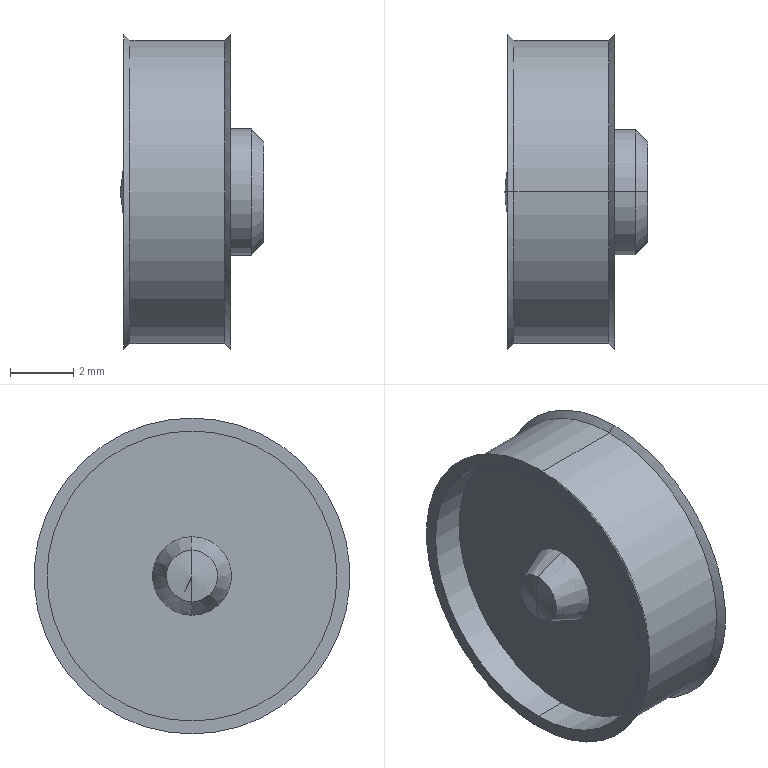Part | SolidWorks | features Revolution 1 | 1 solid | 28 faces | box 4.55 x 10.02 x 10.02 mm | volume 110.565 mm3 | cone 12 | cylinder 10 | plane 6 | commonest cylinder face diameters 9.2 x4 1.5 x2 4 x2 9.62 x2
STEP:
#1=CARTESIAN_POINT('',(-1.243,0.,4.81));
#2=VERTEX_POINT('',#1);
#3=CARTESIAN_POINT('',(-1.243,0.,-4.81));
#4=VERTEX_POINT('',#3);
#5=CARTESIAN_POINT('',(-1.243,0.,0.));
#6=DIRECTION('',(-1.,0.,0.));
#7=DIRECTION('',(0.,0.,1.));
#8=AXIS2_PLACEMENT_3D('',#5,#6,#7);
#9=CIRCLE('',#8,4.81);
#10=EDGE_CURVE('',#2,#4,#9,.T.);
#11=ORIENTED_EDGE('',*,*,#10,.T.);
#12=CARTESIAN_POINT('',(-4.243,0.,-4.81));
#13=VERTEX_POINT('',#12);
#14=CARTESIAN_POINT('',(-2.75,0.,-4.81));
#15=DIRECTION('',(-1.,0.,0.));
#16=VECTOR('',#15,1000.);
#17=LINE('',#14,#16);
#18=EDGE_CURVE('',#4,#13,#17,.T.);
#19=ORIENTED_EDGE('',*,*,#18,.T.);
#20=CARTESIAN_POINT('',(-4.243,0.,4.81));
#21=VERTEX_POINT('',#20);
#22=CARTESIAN_POINT('',(-4.243,0.,0.));
#23=DIRECTION('',(-1.,0.,0.));
#24=DIRECTION('',(0.,0.,1.));
#25=AXIS2_PLACEMENT_3D('',#22,#23,#24);
#26=CIRCLE('',#25,4.81);
#27=EDGE_CURVE('',#21,#13,#26,.T.);
#28=ORIENTED_EDGE('',*,*,#27,.F.);
#29=CARTESIAN_POINT('',(-2.75,0.,4.81));
#30=DIRECTION('',(-1.,0.,0.));
#31=VECTOR('',#30,1000.);
#32=LINE('',#29,#31);
#33=EDGE_CURVE('',#2,#21,#32,.T.);
#34=ORIENTED_EDGE('',*,*,#33,.F.);
#35=EDGE_LOOP('',(#11,#19,#28,#34));
#36=FACE_OUTER_BOUND('',#35,.T.);
#37=CARTESIAN_POINT('',(-2.75,0.,0.));
#38=DIRECTION('',(-1.,0.,0.));
#39=DIRECTION('',(0.,0.,1.));
#40=AXIS2_PLACEMENT_3D('',#37,#38,#39);
#41=CYLINDRICAL_SURFACE('',#40,4.81);
#42=ADVANCED_FACE('',(#36),#41,.T.);
#43=ORIENTED_EDGE('',*,*,#10,.F.);
#44=CARTESIAN_POINT('',(-1.043,0.,5.01));
#45=VERTEX_POINT('',#44);
#46=CARTESIAN_POINT('',(-1.043,0.,5.01));
#47=DIRECTION('',(0.7071,0.,0.7071));
#48=VECTOR('',#47,1000.);
#49=LINE('',#46,#48);
#50=EDGE_CURVE('',#2,#45,#49,.T.);
#51=ORIENTED_EDGE('',*,*,#50,.T.);
#52=CARTESIAN_POINT('',(-1.043,0.,-5.01));
#53=VERTEX_POINT('',#52);
#54=CARTESIAN_POINT('',(-1.043,0.,0.));
#55=DIRECTION('',(-1.,0.,0.));
#56=DIRECTION('',(0.,0.,1.));
#57=AXIS2_PLACEMENT_3D('',#54,#55,#56);
#58=CIRCLE('',#57,5.01);
#59=EDGE_CURVE('',#45,#53,#58,.T.);
#60=ORIENTED_EDGE('',*,*,#59,.T.);
#61=CARTESIAN_POINT('',(-1.043,0.,-5.01));
#62=DIRECTION('',(0.7071,0.,-0.7071));
#63=VECTOR('',#62,1000.);
#64=LINE('',#61,#63);
#65=EDGE_CURVE('',#4,#53,#64,.T.);
#66=ORIENTED_EDGE('',*,*,#65,.F.);
#67=EDGE_LOOP('',(#43,#51,#60,#66));
#68=FACE_OUTER_BOUND('',#67,.T.);
#69=CARTESIAN_POINT('',(-1.043,0.,0.));
#70=DIRECTION('',(1.,0.,0.));
#71=DIRECTION('',(0.,0.,-1.));
#72=AXIS2_PLACEMENT_3D('',#69,#70,#71);
#73=CONICAL_SURFACE('',#72,5.01,0.7854);
#74=ADVANCED_FACE('',(#68),#73,.T.);
#75=CARTESIAN_POINT('',(-1.043,0.,-4.6));
#76=VERTEX_POINT('',#75);
#77=CARTESIAN_POINT('',(-1.043,0.,4.6));
#78=VERTEX_POINT('',#77);
#79=CARTESIAN_POINT('',(-1.043,0.,0.));
#80=DIRECTION('',(-1.,0.,0.));
#81=DIRECTION('',(0.,0.,1.));
#82=AXIS2_PLACEMENT_3D('',#79,#80,#81);
#83=CIRCLE('',#82,4.6);
#84=EDGE_CURVE('',#76,#78,#83,.T.);
#85=ORIENTED_EDGE('',*,*,#84,.F.);
#86=CARTESIAN_POINT('',(-2.643,0.,-4.6));
#87=VERTEX_POINT('',#86);
#88=CARTESIAN_POINT('',(-2.75,0.,-4.6));
#89=DIRECTION('',(-1.,0.,0.));
#90=VECTOR('',#89,1000.);
#91=LINE('',#88,#90);
#92=EDGE_CURVE('',#76,#87,#91,.T.);
#93=ORIENTED_EDGE('',*,*,#92,.T.);
#94=CARTESIAN_POINT('',(-2.643,0.,4.6));
#95=VERTEX_POINT('',#94);
#96=CARTESIAN_POINT('',(-2.643,0.,0.));
#97=DIRECTION('',(-1.,0.,0.));
#98=DIRECTION('',(0.,0.,1.));
#99=AXIS2_PLACEMENT_3D('',#96,#97,#98);
#100=CIRCLE('',#99,4.6);
#101=EDGE_CURVE('',#87,#95,#100,.T.);
#102=ORIENTED_EDGE('',*,*,#101,.T.);
#103=CARTESIAN_POINT('',(-2.75,0.,4.6));
#104=DIRECTION('',(-1.,0.,0.));
#105=VECTOR('',#104,1000.);
#106=LINE('',#103,#105);
#107=EDGE_CURVE('',#78,#95,#106,.T.);
#108=ORIENTED_EDGE('',*,*,#107,.F.);
#109=EDGE_LOOP('',(#85,#93,#102,#108));
#110=FACE_OUTER_BOUND('',#109,.T.);
#111=CARTESIAN_POINT('',(-2.75,0.,0.));
#112=DIRECTION('',(-1.,0.,0.));
#113=DIRECTION('',(0.,0.,1.));
#114=AXIS2_PLACEMENT_3D('',#111,#112,#113);
#115=CYLINDRICAL_SURFACE('',#114,4.6);
#116=ADVANCED_FACE('',(#110),#115,.F.);
#117=CARTESIAN_POINT('',(-1.643,0.,2.));
#118=VERTEX_POINT('',#117);
#119=CARTESIAN_POINT('',(-1.643,0.,-2.));
#120=VERTEX_POINT('',#119);
#121=CARTESIAN_POINT('',(-1.643,0.,0.));
#122=DIRECTION('',(-1.,0.,0.));
#123=DIRECTION('',(0.,0.,1.));
#124=AXIS2_PLACEMENT_3D('',#121,#122,#123);
#125=CIRCLE('',#124,2.);
#126=EDGE_CURVE('',#118,#120,#125,.T.);
#127=ORIENTED_EDGE('',*,*,#126,.T.);
#128=CARTESIAN_POINT('',(-2.643,0.,-3.));
#129=VERTEX_POINT('',#128);
#130=CARTESIAN_POINT('',(-1.643,0.,-2.));
#131=DIRECTION('',(-0.7071,0.,-0.7071));
#132=VECTOR('',#131,1000.);
#133=LINE('',#130,#132);
#134=EDGE_CURVE('',#120,#129,#133,.T.);
#135=ORIENTED_EDGE('',*,*,#134,.T.);
#136=CARTESIAN_POINT('',(-2.643,0.,3.));
#137=VERTEX_POINT('',#136);
#138=CARTESIAN_POINT('',(-2.643,0.,0.));
#139=DIRECTION('',(-1.,0.,0.));
#140=DIRECTION('',(0.,0.,1.));
#141=AXIS2_PLACEMENT_3D('',#138,#139,#140);
#142=CIRCLE('',#141,3.);
#143=EDGE_CURVE('',#137,#129,#142,.T.);
#144=ORIENTED_EDGE('',*,*,#143,.F.);
#145=CARTESIAN_POINT('',(-1.643,0.,2.));
#146=DIRECTION('',(-0.7071,0.,0.7071));
#147=VECTOR('',#146,1000.);
#148=LINE('',#145,#147);
#149=EDGE_CURVE('',#118,#137,#148,.T.);
#150=ORIENTED_EDGE('',*,*,#149,.F.);
#151=EDGE_LOOP('',(#127,#135,#144,#150));
#152=FACE_OUTER_BOUND('',#151,.T.);
#153=CARTESIAN_POINT('',(-1.643,0.,0.));
#154=DIRECTION('',(-1.,0.,0.));
#155=DIRECTION('',(0.,0.,1.));
#156=AXIS2_PLACEMENT_3D('',#153,#154,#155);
#157=CONICAL_SURFACE('',#156,2.,0.7854);
#158=ADVANCED_FACE('',(#152),#157,.T.);
#159=CARTESIAN_POINT('',(-0.4,0.,2.));
#160=VERTEX_POINT('',#159);
#161=CARTESIAN_POINT('',(-0.4,0.,-2.));
#162=VERTEX_POINT('',#161);
#163=CARTESIAN_POINT('',(-0.4,0.,0.));
#164=DIRECTION('',(-1.,0.,0.));
#165=DIRECTION('',(0.,0.,1.));
#166=AXIS2_PLACEMENT_3D('',#163,#164,#165);
#167=CIRCLE('',#166,2.);
#168=EDGE_CURVE('',#160,#162,#167,.T.);
#169=ORIENTED_EDGE('',*,*,#168,.T.);
#170=CARTESIAN_POINT('',(-2.75,0.,-2.));
#171=DIRECTION('',(-1.,0.,0.));
#172=VECTOR('',#171,1000.);
#173=LINE('',#170,#172);
#174=EDGE_CURVE('',#162,#120,#173,.T.);
#175=ORIENTED_EDGE('',*,*,#174,.T.);
#176=ORIENTED_EDGE('',*,*,#126,.F.);
#177=CARTESIAN_POINT('',(-2.75,0.,2.));
#178=DIRECTION('',(-1.,0.,0.));
#179=VECTOR('',#178,1000.);
#180=LINE('',#177,#179);
#181=EDGE_CURVE('',#160,#118,#180,.T.);
#182=ORIENTED_EDGE('',*,*,#181,.F.);
#183=EDGE_LOOP('',(#169,#175,#176,#182));
#184=FACE_OUTER_BOUND('',#183,.T.);
#185=CARTESIAN_POINT('',(-2.75,0.,0.));
#186=DIRECTION('',(-1.,0.,0.));
#187=DIRECTION('',(0.,0.,1.));
#188=AXIS2_PLACEMENT_3D('',#185,#186,#187);
#189=CYLINDRICAL_SURFACE('',#188,2.);
#190=ADVANCED_FACE('',(#184),#189,.T.);
#191=CARTESIAN_POINT('',(0.,0.,1.6));
#192=VERTEX_POINT('',#191);
#193=CARTESIAN_POINT('',(0.,0.,-1.6));
#194=VERTEX_POINT('',#193);
#195=CARTESIAN_POINT('',(0.,0.,0.));
#196=DIRECTION('',(-1.,0.,0.));
#197=DIRECTION('',(0.,0.,1.));
#198=AXIS2_PLACEMENT_3D('',#195,#196,#197);
#199=CIRCLE('',#198,1.6);
#200=EDGE_CURVE('',#192,#194,#199,.T.);
#201=ORIENTED_EDGE('',*,*,#200,.T.);
#202=CARTESIAN_POINT('',(0.,0.,-1.6));
#203=DIRECTION('',(-0.7071,0.,-0.7071));
#204=VECTOR('',#203,1000.);
#205=LINE('',#202,#204);
#206=EDGE_CURVE('',#194,#162,#205,.T.);
#207=ORIENTED_EDGE('',*,*,#206,.T.);
#208=ORIENTED_EDGE('',*,*,#168,.F.);
#209=CARTESIAN_POINT('',(0.,0.,1.6));
#210=DIRECTION('',(-0.7071,0.,0.7071));
#211=VECTOR('',#210,1000.);
#212=LINE('',#209,#211);
#213=EDGE_CURVE('',#192,#160,#212,.T.);
#214=ORIENTED_EDGE('',*,*,#213,.F.);
#215=EDGE_LOOP('',(#201,#207,#208,#214));
#216=FACE_OUTER_BOUND('',#215,.T.);
#217=CARTESIAN_POINT('',(0.,0.,0.));
#218=DIRECTION('',(-1.,0.,0.));
#219=DIRECTION('',(0.,0.,1.));
#220=AXIS2_PLACEMENT_3D('',#217,#218,#219);
#221=CONICAL_SURFACE('',#220,1.6,0.7854);
#222=ADVANCED_FACE('',(#216),#221,.T.);
#223=CARTESIAN_POINT('',(0.,0.,-0.75));
#224=VERTEX_POINT('',#223);
#225=CARTESIAN_POINT('',(0.,0.,0.75));
#226=VERTEX_POINT('',#225);
#227=CARTESIAN_POINT('',(0.,0.,0.));
#228=DIRECTION('',(-1.,0.,0.));
#229=DIRECTION('',(0.,0.,1.));
#230=AXIS2_PLACEMENT_3D('',#227,#228,#229);
#231=CIRCLE('',#230,0.75);
#232=EDGE_CURVE('',#224,#226,#231,.T.);
#233=ORIENTED_EDGE('',*,*,#232,.F.);
#234=CARTESIAN_POINT('',(-2.75,0.,-0.75));
#235=VERTEX_POINT('',#234);
#236=CARTESIAN_POINT('',(-2.75,0.,-0.75));
#237=DIRECTION('',(-1.,0.,0.));
#238=VECTOR('',#237,1000.);
#239=LINE('',#236,#238);
#240=EDGE_CURVE('',#224,#235,#239,.T.);
#241=ORIENTED_EDGE('',*,*,#240,.T.);
#242=CARTESIAN_POINT('',(-2.75,0.,0.75));
#243=VERTEX_POINT('',#242);
#244=CARTESIAN_POINT('',(-2.75,0.,0.));
#245=DIRECTION('',(-1.,0.,0.));
#246=DIRECTION('',(0.,0.,1.));
#247=AXIS2_PLACEMENT_3D('',#244,#245,#246);
#248=CIRCLE('',#247,0.75);
#249=EDGE_CURVE('',#235,#243,#248,.T.);
#250=ORIENTED_EDGE('',*,*,#249,.T.);
#251=CARTESIAN_POINT('',(-2.75,0.,0.75));
#252=DIRECTION('',(-1.,0.,0.));
#253=VECTOR('',#252,1000.);
#254=LINE('',#251,#253);
#255=EDGE_CURVE('',#226,#243,#254,.T.);
#256=ORIENTED_EDGE('',*,*,#255,.F.);
#257=EDGE_LOOP('',(#233,#241,#250,#256));
#258=FACE_OUTER_BOUND('',#257,.T.);
#259=CARTESIAN_POINT('',(-2.75,0.,0.));
#260=DIRECTION('',(-1.,0.,0.));
#261=DIRECTION('',(0.,0.,1.));
#262=AXIS2_PLACEMENT_3D('',#259,#260,#261);
#263=CYLINDRICAL_SURFACE('',#262,0.75);
#264=ADVANCED_FACE('',(#258),#263,.F.);
#265=CARTESIAN_POINT('',(-4.55,0.,0.));
#266=VERTEX_POINT('',#265);
#267=CARTESIAN_POINT('',(-4.443,0.,-0.8131));
#268=VERTEX_POINT('',#267);
#269=CARTESIAN_POINT('',(-4.443,0.,-0.8131));
#270=DIRECTION('',(0.1305,0.,-0.9914));
#271=VECTOR('',#270,1000.);
#272=LINE('',#269,#271);
#273=EDGE_CURVE('',#266,#268,#272,.T.);
#274=ORIENTED_EDGE('',*,*,#273,.F.);
#275=CARTESIAN_POINT('',(-4.443,0.,0.8131));
#276=VERTEX_POINT('',#275);
#277=CARTESIAN_POINT('',(-4.443,0.,0.8131));
#278=DIRECTION('',(0.1305,0.,0.9914));
#279=VECTOR('',#278,1000.);
#280=LINE('',#277,#279);
#281=EDGE_CURVE('',#266,#276,#280,.T.);
#282=ORIENTED_EDGE('',*,*,#281,.T.);
#283=CARTESIAN_POINT('',(-4.443,0.,0.));
#284=DIRECTION('',(-1.,0.,0.));
#285=DIRECTION('',(0.,0.,1.));
#286=AXIS2_PLACEMENT_3D('',#283,#284,#285);
#287=CIRCLE('',#286,0.8131);
#288=EDGE_CURVE('',#276,#268,#287,.T.);
#289=ORIENTED_EDGE('',*,*,#288,.T.);
#290=EDGE_LOOP('',(#274,#282,#289));
#291=FACE_OUTER_BOUND('',#290,.T.);
#292=CARTESIAN_POINT('',(-4.443,0.,0.));
#293=DIRECTION('',(1.,0.,0.));
#294=DIRECTION('',(0.,0.,-1.));
#295=AXIS2_PLACEMENT_3D('',#292,#293,#294);
#296=CONICAL_SURFACE('',#295,0.8131,1.44);
#297=ADVANCED_FACE('',(#291),#296,.T.);
#298=ORIENTED_EDGE('',*,*,#288,.F.);
#299=CARTESIAN_POINT('',(-3.393,0.,1.248));
#300=VERTEX_POINT('',#299);
#301=CARTESIAN_POINT('',(-3.393,0.,1.248));
#302=DIRECTION('',(0.9239,0.,0.3827));
#303=VECTOR('',#302,1000.);
#304=LINE('',#301,#303);
#305=EDGE_CURVE('',#276,#300,#304,.T.);
#306=ORIENTED_EDGE('',*,*,#305,.T.);
#307=CARTESIAN_POINT('',(-3.393,0.,-1.248));
#308=VERTEX_POINT('',#307);
#309=CARTESIAN_POINT('',(-3.393,0.,0.));
#310=DIRECTION('',(-1.,0.,0.));
#311=DIRECTION('',(0.,0.,1.));
#312=AXIS2_PLACEMENT_3D('',#309,#310,#311);
#313=CIRCLE('',#312,1.248);
#314=EDGE_CURVE('',#300,#308,#313,.T.);
#315=ORIENTED_EDGE('',*,*,#314,.T.);
#316=CARTESIAN_POINT('',(-3.393,0.,-1.248));
#317=DIRECTION('',(0.9239,0.,-0.3827));
#318=VECTOR('',#317,1000.);
#319=LINE('',#316,#318);
#320=EDGE_CURVE('',#268,#308,#319,.T.);
#321=ORIENTED_EDGE('',*,*,#320,.F.);
#322=EDGE_LOOP('',(#298,#306,#315,#321));
#323=FACE_OUTER_BOUND('',#322,.T.);
#324=CARTESIAN_POINT('',(-3.393,0.,0.));
#325=DIRECTION('',(1.,0.,0.));
#326=DIRECTION('',(0.,0.,-1.));
#327=AXIS2_PLACEMENT_3D('',#324,#325,#326);
#328=CONICAL_SURFACE('',#327,1.248,0.3927);
#329=ADVANCED_FACE('',(#323),#328,.T.);
#330=CARTESIAN_POINT('',(-3.393,0.,-4.6));
#331=VERTEX_POINT('',#330);
#332=CARTESIAN_POINT('',(-3.393,0.,4.6));
#333=VERTEX_POINT('',#332);
#334=CARTESIAN_POINT('',(-3.393,0.,0.));
#335=DIRECTION('',(-1.,0.,0.));
#336=DIRECTION('',(0.,0.,1.));
#337=AXIS2_PLACEMENT_3D('',#334,#335,#336);
#338=CIRCLE('',#337,4.6);
#339=EDGE_CURVE('',#331,#333,#338,.T.);
#340=ORIENTED_EDGE('',*,*,#339,.F.);
#341=CARTESIAN_POINT('',(-4.443,0.,-4.6));
#342=VERTEX_POINT('',#341);
#343=CARTESIAN_POINT('',(-2.75,0.,-4.6));
#344=DIRECTION('',(-1.,0.,0.));
#345=VECTOR('',#344,1000.);
#346=LINE('',#343,#345);
#347=EDGE_CURVE('',#331,#342,#346,.T.);
#348=ORIENTED_EDGE('',*,*,#347,.T.);
#349=CARTESIAN_POINT('',(-4.443,0.,4.6));
#350=VERTEX_POINT('',#349);
#351=CARTESIAN_POINT('',(-4.443,0.,0.));
#352=DIRECTION('',(-1.,0.,0.));
#353=DIRECTION('',(0.,0.,1.));
#354=AXIS2_PLACEMENT_3D('',#351,#352,#353);
#355=CIRCLE('',#354,4.6);
#356=EDGE_CURVE('',#342,#350,#355,.T.);
#357=ORIENTED_EDGE('',*,*,#356,.T.);
#358=CARTESIAN_POINT('',(-2.75,0.,4.6));
#359=DIRECTION('',(-1.,0.,0.));
#360=VECTOR('',#359,1000.);
#361=LINE('',#358,#360);
#362=EDGE_CURVE('',#333,#350,#361,.T.);
#363=ORIENTED_EDGE('',*,*,#362,.F.);
#364=EDGE_LOOP('',(#340,#348,#357,#363));
#365=FACE_OUTER_BOUND('',#364,.T.);
#366=CARTESIAN_POINT('',(-2.75,0.,0.));
#367=DIRECTION('',(-1.,0.,0.));
#368=DIRECTION('',(0.,0.,1.));
#369=AXIS2_PLACEMENT_3D('',#366,#367,#368);
#370=CYLINDRICAL_SURFACE('',#369,4.6);
#371=ADVANCED_FACE('',(#365),#370,.F.);
#372=ORIENTED_EDGE('',*,*,#27,.T.);
#373=CARTESIAN_POINT('',(-4.443,0.,-5.01));
#374=VERTEX_POINT('',#373);
#375=CARTESIAN_POINT('',(-4.243,0.,-4.81));
#376=DIRECTION('',(-0.7071,0.,-0.7071));
#377=VECTOR('',#376,1000.);
#378=LINE('',#375,#377);
#379=EDGE_CURVE('',#13,#374,#378,.T.);
#380=ORIENTED_EDGE('',*,*,#379,.T.);
#381=CARTESIAN_POINT('',(-4.443,0.,5.01));
#382=VERTEX_POINT('',#381);
#383=CARTESIAN_POINT('',(-4.443,0.,0.));
#384=DIRECTION('',(-1.,0.,0.));
#385=DIRECTION('',(0.,0.,1.));
#386=AXIS2_PLACEMENT_3D('',#383,#384,#385);
#387=CIRCLE('',#386,5.01);
#388=EDGE_CURVE('',#382,#374,#387,.T.);
#389=ORIENTED_EDGE('',*,*,#388,.F.);
#390=CARTESIAN_POINT('',(-4.243,0.,4.81));
#391=DIRECTION('',(-0.7071,0.,0.7071));
#392=VECTOR('',#391,1000.);
#393=LINE('',#390,#392);
#394=EDGE_CURVE('',#21,#382,#393,.T.);
#395=ORIENTED_EDGE('',*,*,#394,.F.);
#396=EDGE_LOOP('',(#372,#380,#389,#395));
#397=FACE_OUTER_BOUND('',#396,.T.);
#398=CARTESIAN_POINT('',(-4.243,0.,0.));
#399=DIRECTION('',(-1.,0.,0.));
#400=DIRECTION('',(0.,0.,1.));
#401=AXIS2_PLACEMENT_3D('',#398,#399,#400);
#402=CONICAL_SURFACE('',#401,4.81,0.7854);
#403=ADVANCED_FACE('',(#397),#402,.T.);
#404=ORIENTED_EDGE('',*,*,#379,.F.);
#405=CARTESIAN_POINT('',(-4.243,0.,0.));
#406=DIRECTION('',(-1.,0.,0.));
#407=DIRECTION('',(0.,0.,1.));
#408=AXIS2_PLACEMENT_3D('',#405,#406,#407);
#409=CIRCLE('',#408,4.81);
#410=EDGE_CURVE('',#13,#21,#409,.T.);
#411=ORIENTED_EDGE('',*,*,#410,.T.);
#412=ORIENTED_EDGE('',*,*,#394,.T.);
#413=CARTESIAN_POINT('',(-4.443,0.,0.));
#414=DIRECTION('',(-1.,0.,0.));
#415=DIRECTION('',(0.,0.,1.));
#416=AXIS2_PLACEMENT_3D('',#413,#414,#415);
#417=CIRCLE('',#416,5.01);
#418=EDGE_CURVE('',#374,#382,#417,.T.);
#419=ORIENTED_EDGE('',*,*,#418,.F.);
#420=EDGE_LOOP('',(#404,#411,#412,#419));
#421=FACE_OUTER_BOUND('',#420,.T.);
#422=CARTESIAN_POINT('',(-4.243,0.,0.));
#423=DIRECTION('',(-1.,0.,0.));
#424=DIRECTION('',(0.,0.,1.));
#425=AXIS2_PLACEMENT_3D('',#422,#423,#424);
#426=CONICAL_SURFACE('',#425,4.81,0.7854);
#427=ADVANCED_FACE('',(#421),#426,.T.);
#428=CARTESIAN_POINT('',(-4.443,0.,0.));
#429=DIRECTION('',(-1.,0.,0.));
#430=DIRECTION('',(0.,0.,1.));
#431=AXIS2_PLACEMENT_3D('',#428,#429,#430);
#432=CIRCLE('',#431,4.6);
#433=EDGE_CURVE('',#350,#342,#432,.T.);
#434=ORIENTED_EDGE('',*,*,#433,.F.);
#435=ORIENTED_EDGE('',*,*,#356,.F.);
#436=EDGE_LOOP('',(#434,#435));
#437=FACE_BOUND('',#436,.T.);
#438=ORIENTED_EDGE('',*,*,#388,.T.);
#439=ORIENTED_EDGE('',*,*,#418,.T.);
#440=EDGE_LOOP('',(#438,#439));
#441=FACE_OUTER_BOUND('',#440,.T.);
#442=CARTESIAN_POINT('',(-4.443,5.01,0.));
#443=DIRECTION('',(1.,0.,0.));
#444=DIRECTION('',(0.,0.,-1.));
#445=AXIS2_PLACEMENT_3D('',#442,#443,#444);
#446=PLANE('',#445);
#447=ADVANCED_FACE('',(#437,#441),#446,.F.);
#448=ORIENTED_EDGE('',*,*,#347,.F.);
#449=CARTESIAN_POINT('',(-3.393,0.,0.));
#450=DIRECTION('',(-1.,0.,0.));
#451=DIRECTION('',(0.,0.,1.));
#452=AXIS2_PLACEMENT_3D('',#449,#450,#451);
#453=CIRCLE('',#452,4.6);
#454=EDGE_CURVE('',#333,#331,#453,.T.);
#455=ORIENTED_EDGE('',*,*,#454,.F.);
#456=ORIENTED_EDGE('',*,*,#362,.T.);
#457=ORIENTED_EDGE('',*,*,#433,.T.);
#458=EDGE_LOOP('',(#448,#455,#456,#457));
#459=FACE_OUTER_BOUND('',#458,.T.);
#460=CARTESIAN_POINT('',(-2.75,0.,0.));
#461=DIRECTION('',(-1.,0.,0.));
#462=DIRECTION('',(0.,0.,1.));
#463=AXIS2_PLACEMENT_3D('',#460,#461,#462);
#464=CYLINDRICAL_SURFACE('',#463,4.6);
#465=ADVANCED_FACE('',(#459),#464,.F.);
#466=CARTESIAN_POINT('',(-3.393,0.,0.));
#467=DIRECTION('',(-1.,0.,0.));
#468=DIRECTION('',(0.,0.,1.));
#469=AXIS2_PLACEMENT_3D('',#466,#467,#468);
#470=CIRCLE('',#469,1.248);
#471=EDGE_CURVE('',#308,#300,#470,.T.);
#472=ORIENTED_EDGE('',*,*,#471,.F.);
#473=ORIENTED_EDGE('',*,*,#314,.F.);
#474=EDGE_LOOP('',(#472,#473));
#475=FACE_BOUND('',#474,.T.);
#476=ORIENTED_EDGE('',*,*,#454,.T.);
#477=ORIENTED_EDGE('',*,*,#339,.T.);
#478=EDGE_LOOP('',(#476,#477));
#479=FACE_OUTER_BOUND('',#478,.T.);
#480=CARTESIAN_POINT('',(-3.393,4.6,0.));
#481=DIRECTION('',(1.,0.,0.));
#482=DIRECTION('',(0.,0.,-1.));
#483=AXIS2_PLACEMENT_3D('',#480,#481,#482);
#484=PLANE('',#483);
#485=ADVANCED_FACE('',(#475,#479),#484,.F.);
#486=ORIENTED_EDGE('',*,*,#305,.F.);
#487=CARTESIAN_POINT('',(-4.443,0.,0.));
#488=DIRECTION('',(-1.,0.,0.));
#489=DIRECTION('',(0.,0.,1.));
#490=AXIS2_PLACEMENT_3D('',#487,#488,#489);
#491=CIRCLE('',#490,0.8131);
#492=EDGE_CURVE('',#268,#276,#491,.T.);
#493=ORIENTED_EDGE('',*,*,#492,.F.);
#494=ORIENTED_EDGE('',*,*,#320,.T.);
#495=ORIENTED_EDGE('',*,*,#471,.T.);
#496=EDGE_LOOP('',(#486,#493,#494,#495));
#497=FACE_OUTER_BOUND('',#496,.T.);
#498=CARTESIAN_POINT('',(-3.393,0.,0.));
#499=DIRECTION('',(1.,0.,0.));
#500=DIRECTION('',(0.,0.,-1.));
#501=AXIS2_PLACEMENT_3D('',#498,#499,#500);
#502=CONICAL_SURFACE('',#501,1.248,0.3927);
#503=ADVANCED_FACE('',(#497),#502,.T.);
#504=ORIENTED_EDGE('',*,*,#281,.F.);
#505=ORIENTED_EDGE('',*,*,#273,.T.);
#506=ORIENTED_EDGE('',*,*,#492,.T.);
#507=EDGE_LOOP('',(#504,#505,#506));
#508=FACE_OUTER_BOUND('',#507,.T.);
#509=CARTESIAN_POINT('',(-4.443,0.,0.));
#510=DIRECTION('',(1.,0.,0.));
#511=DIRECTION('',(0.,0.,-1.));
#512=AXIS2_PLACEMENT_3D('',#509,#510,#511);
#513=CONICAL_SURFACE('',#512,0.8131,1.44);
#514=ADVANCED_FACE('',(#508),#513,.T.);
#515=CARTESIAN_POINT('',(-2.75,0.,0.));
#516=DIRECTION('',(-1.,0.,0.));
#517=DIRECTION('',(0.,0.,1.));
#518=AXIS2_PLACEMENT_3D('',#515,#516,#517);
#519=CIRCLE('',#518,0.75);
#520=EDGE_CURVE('',#243,#235,#519,.T.);
#521=ORIENTED_EDGE('',*,*,#520,.F.);
#522=ORIENTED_EDGE('',*,*,#249,.F.);
#523=EDGE_LOOP('',(#521,#522));
#524=FACE_OUTER_BOUND('',#523,.T.);
#525=CARTESIAN_POINT('',(-2.75,0.75,0.));
#526=DIRECTION('',(-1.,0.,0.));
#527=DIRECTION('',(0.,0.,1.));
#528=AXIS2_PLACEMENT_3D('',#525,#526,#527);
#529=PLANE('',#528);
#530=ADVANCED_FACE('',(#524),#529,.F.);
#531=ORIENTED_EDGE('',*,*,#240,.F.);
#532=CARTESIAN_POINT('',(0.,0.,0.));
#533=DIRECTION('',(-1.,0.,0.));
#534=DIRECTION('',(0.,0.,1.));
#535=AXIS2_PLACEMENT_3D('',#532,#533,#534);
#536=CIRCLE('',#535,0.75);
#537=EDGE_CURVE('',#226,#224,#536,.T.);
#538=ORIENTED_EDGE('',*,*,#537,.F.);
#539=ORIENTED_EDGE('',*,*,#255,.T.);
#540=ORIENTED_EDGE('',*,*,#520,.T.);
#541=EDGE_LOOP('',(#531,#538,#539,#540));
#542=FACE_OUTER_BOUND('',#541,.T.);
#543=CARTESIAN_POINT('',(-2.75,0.,0.));
#544=DIRECTION('',(-1.,0.,0.));
#545=DIRECTION('',(0.,0.,1.));
#546=AXIS2_PLACEMENT_3D('',#543,#544,#545);
#547=CYLINDRICAL_SURFACE('',#546,0.75);
#548=ADVANCED_FACE('',(#542),#547,.F.);
#549=ORIENTED_EDGE('',*,*,#200,.F.);
#550=CARTESIAN_POINT('',(0.,0.,0.));
#551=DIRECTION('',(-1.,0.,0.));
#552=DIRECTION('',(0.,0.,1.));
#553=AXIS2_PLACEMENT_3D('',#550,#551,#552);
#554=CIRCLE('',#553,1.6);
#555=EDGE_CURVE('',#194,#192,#554,.T.);
#556=ORIENTED_EDGE('',*,*,#555,.F.);
#557=EDGE_LOOP('',(#549,#556));
#558=FACE_OUTER_BOUND('',#557,.T.);
#559=ORIENTED_EDGE('',*,*,#537,.T.);
#560=ORIENTED_EDGE('',*,*,#232,.T.);
#561=EDGE_LOOP('',(#559,#560));
#562=FACE_BOUND('',#561,.T.);
#563=CARTESIAN_POINT('',(0.,1.6,0.));
#564=DIRECTION('',(-1.,0.,0.));
#565=DIRECTION('',(0.,0.,1.));
#566=AXIS2_PLACEMENT_3D('',#563,#564,#565);
#567=PLANE('',#566);
#568=ADVANCED_FACE('',(#558,#562),#567,.F.);
#569=ORIENTED_EDGE('',*,*,#206,.F.);
#570=ORIENTED_EDGE('',*,*,#555,.T.);
#571=ORIENTED_EDGE('',*,*,#213,.T.);
#572=CARTESIAN_POINT('',(-0.4,0.,0.));
#573=DIRECTION('',(-1.,0.,0.));
#574=DIRECTION('',(0.,0.,1.));
#575=AXIS2_PLACEMENT_3D('',#572,#573,#574);
#576=CIRCLE('',#575,2.);
#577=EDGE_CURVE('',#162,#160,#576,.T.);
#578=ORIENTED_EDGE('',*,*,#577,.F.);
#579=EDGE_LOOP('',(#569,#570,#571,#578));
#580=FACE_OUTER_BOUND('',#579,.T.);
#581=CARTESIAN_POINT('',(0.,0.,0.));
#582=DIRECTION('',(-1.,0.,0.));
#583=DIRECTION('',(0.,0.,1.));
#584=AXIS2_PLACEMENT_3D('',#581,#582,#583);
#585=CONICAL_SURFACE('',#584,1.6,0.7854);
#586=ADVANCED_FACE('',(#580),#585,.T.);
#587=ORIENTED_EDGE('',*,*,#174,.F.);
#588=ORIENTED_EDGE('',*,*,#577,.T.);
#589=ORIENTED_EDGE('',*,*,#181,.T.);
#590=CARTESIAN_POINT('',(-1.643,0.,0.));
#591=DIRECTION('',(-1.,0.,0.));
#592=DIRECTION('',(0.,0.,1.));
#593=AXIS2_PLACEMENT_3D('',#590,#591,#592);
#594=CIRCLE('',#593,2.);
#595=EDGE_CURVE('',#120,#118,#594,.T.);
#596=ORIENTED_EDGE('',*,*,#595,.F.);
#597=EDGE_LOOP('',(#587,#588,#589,#596));
#598=FACE_OUTER_BOUND('',#597,.T.);
#599=CARTESIAN_POINT('',(-2.75,0.,0.));
#600=DIRECTION('',(-1.,0.,0.));
#601=DIRECTION('',(0.,0.,1.));
#602=AXIS2_PLACEMENT_3D('',#599,#600,#601);
#603=CYLINDRICAL_SURFACE('',#602,2.);
#604=ADVANCED_FACE('',(#598),#603,.T.);
#605=ORIENTED_EDGE('',*,*,#134,.F.);
#606=ORIENTED_EDGE('',*,*,#595,.T.);
#607=ORIENTED_EDGE('',*,*,#149,.T.);
#608=CARTESIAN_POINT('',(-2.643,0.,0.));
#609=DIRECTION('',(-1.,0.,0.));
#610=DIRECTION('',(0.,0.,1.));
#611=AXIS2_PLACEMENT_3D('',#608,#609,#610);
#612=CIRCLE('',#611,3.);
#613=EDGE_CURVE('',#129,#137,#612,.T.);
#614=ORIENTED_EDGE('',*,*,#613,.F.);
#615=EDGE_LOOP('',(#605,#606,#607,#614));
#616=FACE_OUTER_BOUND('',#615,.T.);
#617=CARTESIAN_POINT('',(-1.643,0.,0.));
#618=DIRECTION('',(-1.,0.,0.));
#619=DIRECTION('',(0.,0.,1.));
#620=AXIS2_PLACEMENT_3D('',#617,#618,#619);
#621=CONICAL_SURFACE('',#620,2.,0.7854);
#622=ADVANCED_FACE('',(#616),#621,.T.);
#623=CARTESIAN_POINT('',(-2.643,0.,0.));
#624=DIRECTION('',(-1.,0.,0.));
#625=DIRECTION('',(0.,0.,1.));
#626=AXIS2_PLACEMENT_3D('',#623,#624,#625);
#627=CIRCLE('',#626,4.6);
#628=EDGE_CURVE('',#95,#87,#627,.T.);
#629=ORIENTED_EDGE('',*,*,#628,.F.);
#630=ORIENTED_EDGE('',*,*,#101,.F.);
#631=EDGE_LOOP('',(#629,#630));
#632=FACE_OUTER_BOUND('',#631,.T.);
#633=ORIENTED_EDGE('',*,*,#143,.T.);
#634=ORIENTED_EDGE('',*,*,#613,.T.);
#635=EDGE_LOOP('',(#633,#634));
#636=FACE_BOUND('',#635,.T.);
#637=CARTESIAN_POINT('',(-2.643,4.6,0.));
#638=DIRECTION('',(-1.,0.,0.));
#639=DIRECTION('',(0.,0.,1.));
#640=AXIS2_PLACEMENT_3D('',#637,#638,#639);
#641=PLANE('',#640);
#642=ADVANCED_FACE('',(#632,#636),#641,.F.);
#643=ORIENTED_EDGE('',*,*,#92,.F.);
#644=CARTESIAN_POINT('',(-1.043,0.,0.));
#645=DIRECTION('',(-1.,0.,0.));
#646=DIRECTION('',(0.,0.,1.));
#647=AXIS2_PLACEMENT_3D('',#644,#645,#646);
#648=CIRCLE('',#647,4.6);
#649=EDGE_CURVE('',#78,#76,#648,.T.);
#650=ORIENTED_EDGE('',*,*,#649,.F.);
#651=ORIENTED_EDGE('',*,*,#107,.T.);
#652=ORIENTED_EDGE('',*,*,#628,.T.);
#653=EDGE_LOOP('',(#643,#650,#651,#652));
#654=FACE_OUTER_BOUND('',#653,.T.);
#655=CARTESIAN_POINT('',(-2.75,0.,0.));
#656=DIRECTION('',(-1.,0.,0.));
#657=DIRECTION('',(0.,0.,1.));
#658=AXIS2_PLACEMENT_3D('',#655,#656,#657);
#659=CYLINDRICAL_SURFACE('',#658,4.6);
#660=ADVANCED_FACE('',(#654),#659,.F.);
#661=CARTESIAN_POINT('',(-1.043,0.,0.));
#662=DIRECTION('',(-1.,0.,0.));
#663=DIRECTION('',(0.,0.,1.));
#664=AXIS2_PLACEMENT_3D('',#661,#662,#663);
#665=CIRCLE('',#664,5.01);
#666=EDGE_CURVE('',#53,#45,#665,.T.);
#667=ORIENTED_EDGE('',*,*,#666,.F.);
#668=ORIENTED_EDGE('',*,*,#59,.F.);
#669=EDGE_LOOP('',(#667,#668));
#670=FACE_OUTER_BOUND('',#669,.T.);
#671=ORIENTED_EDGE('',*,*,#649,.T.);
#672=ORIENTED_EDGE('',*,*,#84,.T.);
#673=EDGE_LOOP('',(#671,#672));
#674=FACE_BOUND('',#673,.T.);
#675=CARTESIAN_POINT('',(-1.043,5.01,0.));
#676=DIRECTION('',(-1.,0.,0.));
#677=DIRECTION('',(0.,0.,1.));
#678=AXIS2_PLACEMENT_3D('',#675,#676,#677);
#679=PLANE('',#678);
#680=ADVANCED_FACE('',(#670,#674),#679,.F.);
#681=ORIENTED_EDGE('',*,*,#50,.F.);
#682=CARTESIAN_POINT('',(-1.243,0.,0.));
#683=DIRECTION('',(-1.,0.,0.));
#684=DIRECTION('',(0.,0.,1.));
#685=AXIS2_PLACEMENT_3D('',#682,#683,#684);
#686=CIRCLE('',#685,4.81);
#687=EDGE_CURVE('',#4,#2,#686,.T.);
#688=ORIENTED_EDGE('',*,*,#687,.F.);
#689=ORIENTED_EDGE('',*,*,#65,.T.);
#690=ORIENTED_EDGE('',*,*,#666,.T.);
#691=EDGE_LOOP('',(#681,#688,#689,#690));
#692=FACE_OUTER_BOUND('',#691,.T.);
#693=CARTESIAN_POINT('',(-1.043,0.,0.));
#694=DIRECTION('',(1.,0.,0.));
#695=DIRECTION('',(0.,0.,-1.));
#696=AXIS2_PLACEMENT_3D('',#693,#694,#695);
#697=CONICAL_SURFACE('',#696,5.01,0.7854);
#698=ADVANCED_FACE('',(#692),#697,.T.);
#699=ORIENTED_EDGE('',*,*,#18,.F.);
#700=ORIENTED_EDGE('',*,*,#687,.T.);
#701=ORIENTED_EDGE('',*,*,#33,.T.);
#702=ORIENTED_EDGE('',*,*,#410,.F.);
#703=EDGE_LOOP('',(#699,#700,#701,#702));
#704=FACE_OUTER_BOUND('',#703,.T.);
#705=CARTESIAN_POINT('',(-2.75,0.,0.));
#706=DIRECTION('',(-1.,0.,0.));
#707=DIRECTION('',(0.,0.,1.));
#708=AXIS2_PLACEMENT_3D('',#705,#706,#707);
#709=CYLINDRICAL_SURFACE('',#708,4.81);
#710=ADVANCED_FACE('',(#704),#709,.T.);
#711=CLOSED_SHELL('',(#42,#74,#116,#158,#190,#222,#264,#297,#329,#371,#403,#427,#447,#465,#485,#503,#514,#530,#548,#568,#586,#604,#622,#642,#660,#680,#698,#710));
#712=MANIFOLD_SOLID_BREP('',#711);
#713=CARTESIAN_POINT('',(0.,0.,0.));
#714=DIRECTION('',(0.,0.,1.));
#715=DIRECTION('',(1.,0.,0.));
#716=AXIS2_PLACEMENT_3D('',#713,#714,#715);
#717=(LENGTH_UNIT()NAMED_UNIT(*)SI_UNIT(.MILLI.,.METRE.));
#718=UNCERTAINTY_MEASURE_WITH_UNIT(LENGTH_MEASURE(0.00001),#717,'','');
#719=(NAMED_UNIT(*)PLANE_ANGLE_UNIT()SI_UNIT($,.RADIAN.));
#720=(NAMED_UNIT(*)SI_UNIT($,.STERADIAN.)SOLID_ANGLE_UNIT());
#721=(GEOMETRIC_REPRESENTATION_CONTEXT(3)GLOBAL_UNCERTAINTY_ASSIGNED_CONTEXT((#718))GLOBAL_UNIT_ASSIGNED_CONTEXT((#717,#719,#720))REPRESENTATION_CONTEXT('',''));
#722=ADVANCED_BREP_SHAPE_REPRESENTATION('',(#712,#716),#721);